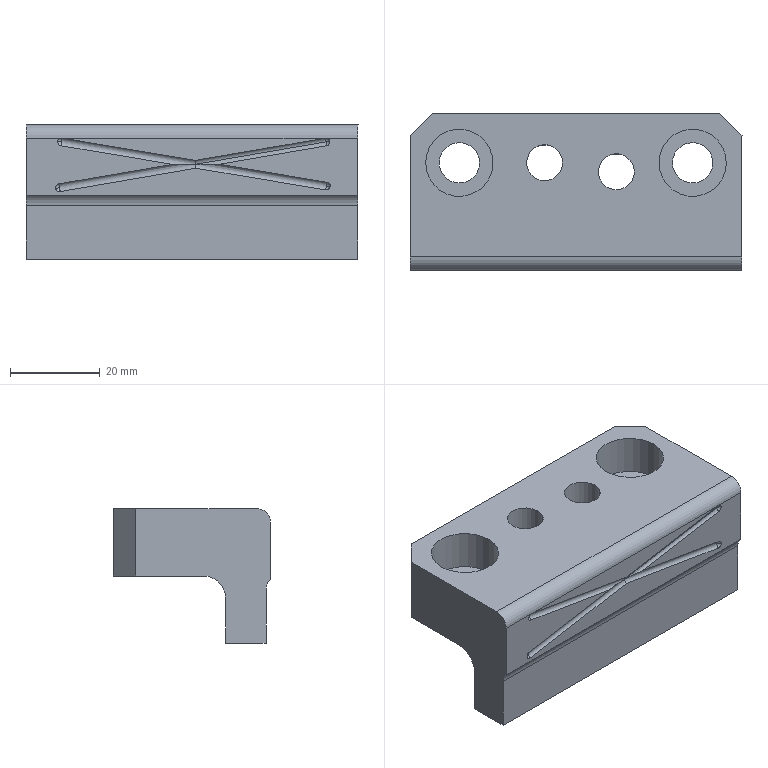Part | CATIA | 1 solid | 42 faces | box 74 x 35 x 30 mm | volume 43302 mm3 | cylinder 20 | plane 14 | sphere 8 | commonest cylinder face diameters 2 x5 8 x4 9 x4 15 x4 6 x2 10 x1
STEP:
#1=CARTESIAN_POINT('',(-37.,5.,-15.));
#2=VERTEX_POINT('',#1);
#3=CARTESIAN_POINT('',(37.,5.,-15.));
#4=VERTEX_POINT('',#3);
#5=CARTESIAN_POINT('',(0.,5.,-15.));
#6=DIRECTION('',(1.,0.,0.));
#7=VECTOR('',#6,1.);
#8=LINE('',#5,#7);
#9=EDGE_CURVE('',#2,#4,#8,.T.);
#10=ORIENTED_EDGE('',*,*,#9,.T.);
#11=CARTESIAN_POINT('',(37.,0.,-20.));
#12=VERTEX_POINT('',#11);
#13=CARTESIAN_POINT('',(37.,5.,-20.));
#14=DIRECTION('',(1.,0.,0.));
#15=AXIS2_PLACEMENT_3D('',#13,#14,$);
#16=CIRCLE('',#15,5.);
#17=EDGE_CURVE('',#4,#12,#16,.T.);
#18=ORIENTED_EDGE('',*,*,#17,.T.);
#19=CARTESIAN_POINT('',(-37.,0.,-20.));
#20=VERTEX_POINT('',#19);
#21=CARTESIAN_POINT('',(0.,0.,-20.));
#22=DIRECTION('',(1.,0.,0.));
#23=VECTOR('',#22,1.);
#24=LINE('',#21,#23);
#25=EDGE_CURVE('',#20,#12,#24,.T.);
#26=ORIENTED_EDGE('',*,*,#25,.F.);
#27=CARTESIAN_POINT('',(-37.,5.,-20.));
#28=DIRECTION('',(1.,0.,0.));
#29=AXIS2_PLACEMENT_3D('',#27,#28,$);
#30=CIRCLE('',#29,5.);
#31=EDGE_CURVE('',#20,#2,#30,.F.);
#32=ORIENTED_EDGE('',*,*,#31,.T.);
#33=EDGE_LOOP('',(#10,#18,#26,#32));
#34=FACE_OUTER_BOUND('',#33,.T.);
#35=CARTESIAN_POINT('',(0.,5.,-20.));
#36=DIRECTION('',(1.,0.,0.));
#37=DIRECTION('',(0.,0.,1.));
#38=AXIS2_PLACEMENT_3D('',#35,#36,#37);
#39=CYLINDRICAL_SURFACE('',#38,5.);
#40=ADVANCED_FACE('',(#34),#39,.F.);
#41=CARTESIAN_POINT('',(-37.,0.,-30.));
#42=VERTEX_POINT('',#41);
#43=CARTESIAN_POINT('',(-37.,0.,-25.));
#44=DIRECTION('',(0.,0.,1.));
#45=VECTOR('',#44,1.);
#46=LINE('',#43,#45);
#47=EDGE_CURVE('',#42,#20,#46,.T.);
#48=ORIENTED_EDGE('',*,*,#47,.T.);
#49=ORIENTED_EDGE('',*,*,#25,.T.);
#50=CARTESIAN_POINT('',(37.,0.,-30.));
#51=VERTEX_POINT('',#50);
#52=CARTESIAN_POINT('',(37.,0.,-25.));
#53=DIRECTION('',(0.,0.,1.));
#54=VECTOR('',#53,1.);
#55=LINE('',#52,#54);
#56=EDGE_CURVE('',#51,#12,#55,.T.);
#57=ORIENTED_EDGE('',*,*,#56,.F.);
#58=CARTESIAN_POINT('',(0.,0.,-30.));
#59=DIRECTION('',(1.,0.,0.));
#60=VECTOR('',#59,1.);
#61=LINE('',#58,#60);
#62=EDGE_CURVE('',#42,#51,#61,.T.);
#63=ORIENTED_EDGE('',*,*,#62,.F.);
#64=EDGE_LOOP('',(#48,#49,#57,#63));
#65=FACE_OUTER_BOUND('',#64,.T.);
#66=CARTESIAN_POINT('',(0.,0.,-30.));
#67=DIRECTION('',(0.,1.,0.));
#68=DIRECTION('',(0.,0.,1.));
#69=AXIS2_PLACEMENT_3D('',#66,#67,#68);
#70=PLANE('',#69);
#71=ADVANCED_FACE('',(#65),#70,.T.);
#72=CARTESIAN_POINT('',(-37.,-9.,-30.));
#73=VERTEX_POINT('',#72);
#74=CARTESIAN_POINT('',(-37.,-4.5,-30.));
#75=DIRECTION('',(0.,1.,0.));
#76=VECTOR('',#75,1.);
#77=LINE('',#74,#76);
#78=EDGE_CURVE('',#73,#42,#77,.T.);
#79=ORIENTED_EDGE('',*,*,#78,.T.);
#80=ORIENTED_EDGE('',*,*,#62,.T.);
#81=CARTESIAN_POINT('',(37.,-9.,-30.));
#82=VERTEX_POINT('',#81);
#83=CARTESIAN_POINT('',(37.,-4.5,-30.));
#84=DIRECTION('',(0.,1.,0.));
#85=VECTOR('',#84,1.);
#86=LINE('',#83,#85);
#87=EDGE_CURVE('',#82,#51,#86,.T.);
#88=ORIENTED_EDGE('',*,*,#87,.F.);
#89=CARTESIAN_POINT('',(0.,-9.,-30.));
#90=DIRECTION('',(1.,0.,0.));
#91=VECTOR('',#90,1.);
#92=LINE('',#89,#91);
#93=EDGE_CURVE('',#73,#82,#92,.T.);
#94=ORIENTED_EDGE('',*,*,#93,.F.);
#95=EDGE_LOOP('',(#79,#80,#88,#94));
#96=FACE_OUTER_BOUND('',#95,.T.);
#97=CARTESIAN_POINT('',(0.,-9.,-30.));
#98=DIRECTION('',(0.,0.,-1.));
#99=DIRECTION('',(0.,1.,0.));
#100=AXIS2_PLACEMENT_3D('',#97,#98,#99);
#101=PLANE('',#100);
#102=ADVANCED_FACE('',(#96),#101,.T.);
#103=CARTESIAN_POINT('',(-37.,-9.,-18.));
#104=VERTEX_POINT('',#103);
#105=CARTESIAN_POINT('',(-37.,-9.,-24.));
#106=DIRECTION('',(0.,0.,-1.));
#107=VECTOR('',#106,1.);
#108=LINE('',#105,#107);
#109=EDGE_CURVE('',#104,#73,#108,.T.);
#110=ORIENTED_EDGE('',*,*,#109,.T.);
#111=ORIENTED_EDGE('',*,*,#93,.T.);
#112=CARTESIAN_POINT('',(37.,-9.,-18.));
#113=VERTEX_POINT('',#112);
#114=CARTESIAN_POINT('',(37.,-9.,-24.));
#115=DIRECTION('',(0.,0.,-1.));
#116=VECTOR('',#115,1.);
#117=LINE('',#114,#116);
#118=EDGE_CURVE('',#113,#82,#117,.T.);
#119=ORIENTED_EDGE('',*,*,#118,.F.);
#120=CARTESIAN_POINT('',(0.,-9.,-18.));
#121=DIRECTION('',(1.,0.,0.));
#122=VECTOR('',#121,1.);
#123=LINE('',#120,#122);
#124=EDGE_CURVE('',#104,#113,#123,.T.);
#125=ORIENTED_EDGE('',*,*,#124,.F.);
#126=EDGE_LOOP('',(#110,#111,#119,#125));
#127=FACE_OUTER_BOUND('',#126,.T.);
#128=CARTESIAN_POINT('',(0.,-9.,-18.));
#129=DIRECTION('',(0.,-1.,0.));
#130=DIRECTION('',(0.,0.,-1.));
#131=AXIS2_PLACEMENT_3D('',#128,#129,#130);
#132=PLANE('',#131);
#133=ADVANCED_FACE('',(#127),#132,.T.);
#134=ORIENTED_EDGE('',*,*,#124,.T.);
#135=CARTESIAN_POINT('',(37.,-10.,-15.764));
#136=VERTEX_POINT('',#135);
#137=CARTESIAN_POINT('',(37.,-12.,-18.));
#138=DIRECTION('',(1.,0.,0.));
#139=AXIS2_PLACEMENT_3D('',#137,#138,$);
#140=CIRCLE('',#139,3.);
#141=EDGE_CURVE('',#113,#136,#140,.T.);
#142=ORIENTED_EDGE('',*,*,#141,.T.);
#143=CARTESIAN_POINT('',(-37.,-10.,-15.764));
#144=VERTEX_POINT('',#143);
#145=CARTESIAN_POINT('',(0.,-10.,-15.764));
#146=DIRECTION('',(1.,0.,0.));
#147=VECTOR('',#146,1.);
#148=LINE('',#145,#147);
#149=EDGE_CURVE('',#144,#136,#148,.T.);
#150=ORIENTED_EDGE('',*,*,#149,.F.);
#151=CARTESIAN_POINT('',(-37.,-12.,-18.));
#152=DIRECTION('',(1.,0.,0.));
#153=AXIS2_PLACEMENT_3D('',#151,#152,$);
#154=CIRCLE('',#153,3.);
#155=EDGE_CURVE('',#144,#104,#154,.F.);
#156=ORIENTED_EDGE('',*,*,#155,.T.);
#157=EDGE_LOOP('',(#134,#142,#150,#156));
#158=FACE_OUTER_BOUND('',#157,.T.);
#159=CARTESIAN_POINT('',(0.,-12.,-18.));
#160=DIRECTION('',(1.,0.,0.));
#161=DIRECTION('',(0.,1.,0.));
#162=AXIS2_PLACEMENT_3D('',#159,#160,#161);
#163=CYLINDRICAL_SURFACE('',#162,3.);
#164=ADVANCED_FACE('',(#158),#163,.F.);
#165=CARTESIAN_POINT('',(37.,20.,0.));
#166=VERTEX_POINT('',#165);
#167=CARTESIAN_POINT('',(37.,-7.,0.));
#168=VERTEX_POINT('',#167);
#169=CARTESIAN_POINT('',(37.,6.5,0.));
#170=DIRECTION('',(0.,-1.,0.));
#171=VECTOR('',#170,1.);
#172=LINE('',#169,#171);
#173=EDGE_CURVE('',#166,#168,#172,.T.);
#174=ORIENTED_EDGE('',*,*,#173,.T.);
#175=CARTESIAN_POINT('',(37.,-10.,-3.));
#176=VERTEX_POINT('',#175);
#177=CARTESIAN_POINT('',(37.,-7.,-3.));
#178=DIRECTION('',(1.,0.,0.));
#179=AXIS2_PLACEMENT_3D('',#177,#178,$);
#180=CIRCLE('',#179,3.);
#181=EDGE_CURVE('',#168,#176,#180,.T.);
#182=ORIENTED_EDGE('',*,*,#181,.T.);
#183=CARTESIAN_POINT('',(37.,-10.,-9.382));
#184=DIRECTION('',(0.,0.,1.));
#185=VECTOR('',#184,1.);
#186=LINE('',#183,#185);
#187=EDGE_CURVE('',#136,#176,#186,.T.);
#188=ORIENTED_EDGE('',*,*,#187,.F.);
#189=ORIENTED_EDGE('',*,*,#141,.F.);
#190=ORIENTED_EDGE('',*,*,#118,.T.);
#191=ORIENTED_EDGE('',*,*,#87,.T.);
#192=ORIENTED_EDGE('',*,*,#56,.T.);
#193=ORIENTED_EDGE('',*,*,#17,.F.);
#194=CARTESIAN_POINT('',(37.,20.,-15.));
#195=VERTEX_POINT('',#194);
#196=CARTESIAN_POINT('',(37.,12.5,-15.));
#197=DIRECTION('',(0.,-1.,0.));
#198=VECTOR('',#197,1.);
#199=LINE('',#196,#198);
#200=EDGE_CURVE('',#195,#4,#199,.T.);
#201=ORIENTED_EDGE('',*,*,#200,.F.);
#202=CARTESIAN_POINT('',(37.,20.,-7.5));
#203=DIRECTION('',(0.,0.,-1.));
#204=VECTOR('',#203,1.);
#205=LINE('',#202,#204);
#206=EDGE_CURVE('',#195,#166,#205,.F.);
#207=ORIENTED_EDGE('',*,*,#206,.T.);
#208=EDGE_LOOP('',(#174,#182,#188,#189,#190,#191,#192,#193,#201,#207));
#209=FACE_OUTER_BOUND('',#208,.T.);
#210=CARTESIAN_POINT('',(37.,-10.,0.));
#211=DIRECTION('',(1.,0.,0.));
#212=DIRECTION('',(0.,1.,0.));
#213=AXIS2_PLACEMENT_3D('',#210,#211,#212);
#214=PLANE('',#213);
#215=ADVANCED_FACE('',(#209),#214,.T.);
#216=ORIENTED_EDGE('',*,*,#206,.F.);
#217=CARTESIAN_POINT('',(32.,25.,-15.));
#218=VERTEX_POINT('',#217);
#219=CARTESIAN_POINT('',(34.5,22.5,-15.));
#220=DIRECTION('',(0.7071,-0.7071,0.));
#221=VECTOR('',#220,1.);
#222=LINE('',#219,#221);
#223=EDGE_CURVE('',#195,#218,#222,.F.);
#224=ORIENTED_EDGE('',*,*,#223,.T.);
#225=CARTESIAN_POINT('',(32.,25.,0.));
#226=VERTEX_POINT('',#225);
#227=CARTESIAN_POINT('',(32.,25.,-15.));
#228=DIRECTION('',(0.,0.,-1.));
#229=VECTOR('',#228,1.);
#230=LINE('',#227,#229);
#231=EDGE_CURVE('',#218,#226,#230,.F.);
#232=ORIENTED_EDGE('',*,*,#231,.T.);
#233=CARTESIAN_POINT('',(34.5,22.5,0.));
#234=DIRECTION('',(0.7071,-0.7071,0.));
#235=VECTOR('',#234,1.);
#236=LINE('',#233,#235);
#237=EDGE_CURVE('',#226,#166,#236,.T.);
#238=ORIENTED_EDGE('',*,*,#237,.T.);
#239=EDGE_LOOP('',(#216,#224,#232,#238));
#240=FACE_OUTER_BOUND('',#239,.T.);
#241=CARTESIAN_POINT('',(32.,25.,6.));
#242=DIRECTION('',(-0.7071,-0.7071,0.));
#243=DIRECTION('',(0.,0.,-1.));
#244=AXIS2_PLACEMENT_3D('',#241,#242,#243);
#245=PLANE('',#244);
#246=ADVANCED_FACE('',(#240),#245,.F.);
#247=CARTESIAN_POINT('',(-37.,20.,-15.));
#248=VERTEX_POINT('',#247);
#249=CARTESIAN_POINT('',(-37.,12.5,-15.));
#250=DIRECTION('',(0.,-1.,0.));
#251=VECTOR('',#250,1.);
#252=LINE('',#249,#251);
#253=EDGE_CURVE('',#248,#2,#252,.T.);
#254=ORIENTED_EDGE('',*,*,#253,.T.);
#255=ORIENTED_EDGE('',*,*,#31,.F.);
#256=ORIENTED_EDGE('',*,*,#47,.F.);
#257=ORIENTED_EDGE('',*,*,#78,.F.);
#258=ORIENTED_EDGE('',*,*,#109,.F.);
#259=ORIENTED_EDGE('',*,*,#155,.F.);
#260=CARTESIAN_POINT('',(-37.,-10.,-3.));
#261=VERTEX_POINT('',#260);
#262=CARTESIAN_POINT('',(-37.,-10.,-9.382));
#263=DIRECTION('',(0.,0.,1.));
#264=VECTOR('',#263,1.);
#265=LINE('',#262,#264);
#266=EDGE_CURVE('',#144,#261,#265,.T.);
#267=ORIENTED_EDGE('',*,*,#266,.T.);
#268=CARTESIAN_POINT('',(-37.,-7.,0.));
#269=VERTEX_POINT('',#268);
#270=CARTESIAN_POINT('',(-37.,-7.,-3.));
#271=DIRECTION('',(-1.,0.,0.));
#272=AXIS2_PLACEMENT_3D('',#270,#271,$);
#273=CIRCLE('',#272,3.);
#274=EDGE_CURVE('',#261,#269,#273,.T.);
#275=ORIENTED_EDGE('',*,*,#274,.T.);
#276=CARTESIAN_POINT('',(-37.,20.,0.));
#277=VERTEX_POINT('',#276);
#278=CARTESIAN_POINT('',(-37.,6.5,0.));
#279=DIRECTION('',(0.,-1.,0.));
#280=VECTOR('',#279,1.);
#281=LINE('',#278,#280);
#282=EDGE_CURVE('',#277,#269,#281,.T.);
#283=ORIENTED_EDGE('',*,*,#282,.F.);
#284=CARTESIAN_POINT('',(-37.,20.,-7.5));
#285=DIRECTION('',(0.,0.,1.));
#286=VECTOR('',#285,1.);
#287=LINE('',#284,#286);
#288=EDGE_CURVE('',#248,#277,#287,.T.);
#289=ORIENTED_EDGE('',*,*,#288,.F.);
#290=EDGE_LOOP('',(#254,#255,#256,#257,#258,#259,#267,#275,#283,#289));
#291=FACE_OUTER_BOUND('',#290,.T.);
#292=CARTESIAN_POINT('',(-37.,25.,0.));
#293=DIRECTION('',(-1.,0.,0.));
#294=DIRECTION('',(0.,-1.,0.));
#295=AXIS2_PLACEMENT_3D('',#292,#293,#294);
#296=PLANE('',#295);
#297=ADVANCED_FACE('',(#291),#296,.T.);
#298=CARTESIAN_POINT('',(-32.,25.,0.));
#299=VERTEX_POINT('',#298);
#300=CARTESIAN_POINT('',(0.,25.,0.));
#301=DIRECTION('',(1.,0.,0.));
#302=VECTOR('',#301,1.);
#303=LINE('',#300,#302);
#304=EDGE_CURVE('',#299,#226,#303,.T.);
#305=ORIENTED_EDGE('',*,*,#304,.T.);
#306=ORIENTED_EDGE('',*,*,#231,.F.);
#307=CARTESIAN_POINT('',(-32.,25.,-15.));
#308=VERTEX_POINT('',#307);
#309=CARTESIAN_POINT('',(0.,25.,-15.));
#310=DIRECTION('',(1.,0.,0.));
#311=VECTOR('',#310,1.);
#312=LINE('',#309,#311);
#313=EDGE_CURVE('',#308,#218,#312,.T.);
#314=ORIENTED_EDGE('',*,*,#313,.F.);
#315=CARTESIAN_POINT('',(-32.,25.,-7.5));
#316=DIRECTION('',(0.,0.,1.));
#317=VECTOR('',#316,1.);
#318=LINE('',#315,#317);
#319=EDGE_CURVE('',#308,#299,#318,.T.);
#320=ORIENTED_EDGE('',*,*,#319,.T.);
#321=EDGE_LOOP('',(#305,#306,#314,#320));
#322=FACE_OUTER_BOUND('',#321,.T.);
#323=CARTESIAN_POINT('',(0.,25.,-15.));
#324=DIRECTION('',(0.,1.,0.));
#325=DIRECTION('',(0.,0.,1.));
#326=AXIS2_PLACEMENT_3D('',#323,#324,#325);
#327=PLANE('',#326);
#328=ADVANCED_FACE('',(#322),#327,.T.);
#329=ORIENTED_EDGE('',*,*,#319,.F.);
#330=CARTESIAN_POINT('',(-34.5,22.5,-15.));
#331=DIRECTION('',(-0.7071,-0.7071,0.));
#332=VECTOR('',#331,1.);
#333=LINE('',#330,#332);
#334=EDGE_CURVE('',#308,#248,#333,.T.);
#335=ORIENTED_EDGE('',*,*,#334,.T.);
#336=ORIENTED_EDGE('',*,*,#288,.T.);
#337=CARTESIAN_POINT('',(-34.5,22.5,0.));
#338=DIRECTION('',(-0.7071,-0.7071,0.));
#339=VECTOR('',#338,1.);
#340=LINE('',#337,#339);
#341=EDGE_CURVE('',#277,#299,#340,.F.);
#342=ORIENTED_EDGE('',*,*,#341,.T.);
#343=EDGE_LOOP('',(#329,#335,#336,#342));
#344=FACE_OUTER_BOUND('',#343,.T.);
#345=CARTESIAN_POINT('',(-32.,25.,-36.));
#346=DIRECTION('',(0.7071,-0.7071,0.));
#347=DIRECTION('',(0.,0.,1.));
#348=AXIS2_PLACEMENT_3D('',#345,#346,#347);
#349=PLANE('',#348);
#350=ADVANCED_FACE('',(#344),#349,.F.);
#351=CARTESIAN_POINT('',(-28.849,-10.,-3.));
#352=VERTEX_POINT('',#351);
#353=CARTESIAN_POINT('',(29.662,-10.,-3.));
#354=VERTEX_POINT('',#353);
#355=CARTESIAN_POINT('',(0.4066,-10.,-3.));
#356=DIRECTION('',(1.,0.,0.));
#357=VECTOR('',#356,1.);
#358=LINE('',#355,#357);
#359=EDGE_CURVE('',#352,#354,#358,.T.);
#360=ORIENTED_EDGE('',*,*,#359,.F.);
#361=CARTESIAN_POINT('',(0.8431,-10.,-7.948));
#362=VERTEX_POINT('',#361);
#363=CARTESIAN_POINT('',(-14.003,-10.,-5.474));
#364=DIRECTION('',(-0.9864,0.,0.1644));
#365=VECTOR('',#364,1.);
#366=LINE('',#363,#365);
#367=EDGE_CURVE('',#362,#352,#366,.T.);
#368=ORIENTED_EDGE('',*,*,#367,.F.);
#369=CARTESIAN_POINT('',(15.253,-10.,-5.474));
#370=DIRECTION('',(0.9856,0.,0.1692));
#371=VECTOR('',#370,1.);
#372=LINE('',#369,#371);
#373=EDGE_CURVE('',#362,#354,#372,.T.);
#374=ORIENTED_EDGE('',*,*,#373,.T.);
#375=EDGE_LOOP('',(#360,#368,#374));
#376=FACE_OUTER_BOUND('',#375,.T.);
#377=CARTESIAN_POINT('',(0.,-10.,-3.));
#378=DIRECTION('',(0.,-1.,0.));
#379=DIRECTION('',(0.,0.,-1.));
#380=AXIS2_PLACEMENT_3D('',#377,#378,#379);
#381=PLANE('',#380);
#382=ADVANCED_FACE('',(#376),#381,.T.);
#383=CARTESIAN_POINT('',(-29.295,-10.,-3.));
#384=VERTEX_POINT('',#383);
#385=CARTESIAN_POINT('',(-33.147,-10.,-3.));
#386=DIRECTION('',(1.,0.,0.));
#387=VECTOR('',#386,1.);
#388=LINE('',#385,#387);
#389=EDGE_CURVE('',#261,#384,#388,.T.);
#390=ORIENTED_EDGE('',*,*,#389,.F.);
#391=ORIENTED_EDGE('',*,*,#266,.F.);
#392=ORIENTED_EDGE('',*,*,#149,.T.);
#393=ORIENTED_EDGE('',*,*,#187,.T.);
#394=CARTESIAN_POINT('',(30.057,-10.,-3.));
#395=VERTEX_POINT('',#394);
#396=CARTESIAN_POINT('',(33.528,-10.,-3.));
#397=DIRECTION('',(1.,0.,0.));
#398=VECTOR('',#397,1.);
#399=LINE('',#396,#398);
#400=EDGE_CURVE('',#395,#176,#399,.T.);
#401=ORIENTED_EDGE('',*,*,#400,.F.);
#402=CARTESIAN_POINT('',(30.717,-10.,-3.698));
#403=VERTEX_POINT('',#402);
#404=CARTESIAN_POINT('',(30.717,-10.,-3.698));
#405=CARTESIAN_POINT('',(30.701,-10.,-3.603));
#406=CARTESIAN_POINT('',(30.672,-10.,-3.511));
#407=CARTESIAN_POINT('',(30.63,-10.,-3.424));
#408=CARTESIAN_POINT('',(30.558,-10.,-3.315));
#409=CARTESIAN_POINT('',(30.468,-10.,-3.223));
#410=CARTESIAN_POINT('',(30.444,-10.,-3.2));
#411=CARTESIAN_POINT('',(30.36,-10.,-3.129));
#412=CARTESIAN_POINT('',(30.268,-10.,-3.073));
#413=CARTESIAN_POINT('',(30.201,-10.,-3.042));
#414=CARTESIAN_POINT('',(30.132,-10.,-3.018));
#415=CARTESIAN_POINT('',(30.067,-10.,-3.002));
#416=CARTESIAN_POINT('',(30.064,-10.,-3.002));
#417=CARTESIAN_POINT('',(30.06,-10.,-3.001));
#418=CARTESIAN_POINT('',(30.057,-10.,-3.));
#419=B_SPLINE_CURVE_WITH_KNOTS('',5,(#404,#405,#406,#407,#408,#409,#410,#411,#412,#413,#414,#415,#416,#417,#418),.UNSPECIFIED.,.F.,.U.,(6,3,3,3,6),(0.,0.6764,0.913,1.466,1.496),.UNSPECIFIED.);
#420=EDGE_CURVE('',#403,#395,#419,.T.);
#421=ORIENTED_EDGE('',*,*,#420,.F.);
#422=CARTESIAN_POINT('',(30.01,-10.,-4.698));
#423=VERTEX_POINT('',#422);
#424=CARTESIAN_POINT('',(30.01,-10.,-4.698));
#425=CARTESIAN_POINT('',(30.057,-10.,-4.69));
#426=CARTESIAN_POINT('',(30.104,-10.,-4.678));
#427=CARTESIAN_POINT('',(30.152,-10.,-4.663));
#428=CARTESIAN_POINT('',(30.24,-10.,-4.629));
#429=CARTESIAN_POINT('',(30.332,-10.,-4.575));
#430=CARTESIAN_POINT('',(30.373,-10.,-4.547));
#431=CARTESIAN_POINT('',(30.442,-10.,-4.493));
#432=CARTESIAN_POINT('',(30.507,-10.,-4.425));
#433=CARTESIAN_POINT('',(30.532,-10.,-4.397));
#434=CARTESIAN_POINT('',(30.598,-10.,-4.312));
#435=CARTESIAN_POINT('',(30.651,-10.,-4.216));
#436=CARTESIAN_POINT('',(30.678,-10.,-4.151));
#437=CARTESIAN_POINT('',(30.718,-10.,-4.022));
#438=CARTESIAN_POINT('',(30.732,-10.,-3.888));
#439=CARTESIAN_POINT('',(30.733,-10.,-3.824));
#440=CARTESIAN_POINT('',(30.728,-10.,-3.76));
#441=CARTESIAN_POINT('',(30.717,-10.,-3.698));
#442=B_SPLINE_CURVE_WITH_KNOTS('',5,(#424,#425,#426,#427,#428,#429,#430,#431,#432,#433,#434,#435,#436,#437,#438,#439,#440,#441),.UNSPECIFIED.,.F.,.U.,(6,3,3,3,3,6),(0.,0.5372,0.9589,1.243,1.741,2.191),.UNSPECIFIED.);
#443=EDGE_CURVE('',#423,#403,#442,.T.);
#444=ORIENTED_EDGE('',*,*,#443,.F.);
#445=CARTESIAN_POINT('',(6.037,-10.,-8.814));
#446=VERTEX_POINT('',#445);
#447=CARTESIAN_POINT('',(18.024,-10.,-6.756));
#448=DIRECTION('',(-0.9856,0.,-0.1692));
#449=VECTOR('',#448,1.);
#450=LINE('',#447,#449);
#451=EDGE_CURVE('',#423,#446,#450,.T.);
#452=ORIENTED_EDGE('',*,*,#451,.T.);
#453=CARTESIAN_POINT('',(30.078,-10.,-12.821));
#454=VERTEX_POINT('',#453);
#455=CARTESIAN_POINT('',(18.058,-10.,-10.817));
#456=DIRECTION('',(0.9864,0.,-0.1644));
#457=VECTOR('',#456,1.);
#458=LINE('',#455,#457);
#459=EDGE_CURVE('',#446,#454,#458,.T.);
#460=ORIENTED_EDGE('',*,*,#459,.T.);
#461=CARTESIAN_POINT('',(30.79,-10.,-13.817));
#462=VERTEX_POINT('',#461);
#463=CARTESIAN_POINT('',(30.078,-10.,-12.821));
#464=CARTESIAN_POINT('',(30.126,-10.,-12.829));
#465=CARTESIAN_POINT('',(30.173,-10.,-12.84));
#466=CARTESIAN_POINT('',(30.22,-10.,-12.855));
#467=CARTESIAN_POINT('',(30.308,-10.,-12.889));
#468=CARTESIAN_POINT('',(30.401,-10.,-12.942));
#469=CARTESIAN_POINT('',(30.442,-10.,-12.969));
#470=CARTESIAN_POINT('',(30.512,-10.,-13.024));
#471=CARTESIAN_POINT('',(30.577,-10.,-13.091));
#472=CARTESIAN_POINT('',(30.602,-10.,-13.119));
#473=CARTESIAN_POINT('',(30.668,-10.,-13.204));
#474=CARTESIAN_POINT('',(30.721,-10.,-13.3));
#475=CARTESIAN_POINT('',(30.749,-10.,-13.365));
#476=CARTESIAN_POINT('',(30.789,-10.,-13.493));
#477=CARTESIAN_POINT('',(30.804,-10.,-13.627));
#478=CARTESIAN_POINT('',(30.806,-10.,-13.691));
#479=CARTESIAN_POINT('',(30.801,-10.,-13.755));
#480=CARTESIAN_POINT('',(30.79,-10.,-13.817));
#481=B_SPLINE_CURVE_WITH_KNOTS('',5,(#463,#464,#465,#466,#467,#468,#469,#470,#471,#472,#473,#474,#475,#476,#477,#478,#479,#480),.UNSPECIFIED.,.F.,.U.,(6,3,3,3,3,6),(0.,0.5372,0.9589,1.243,1.741,2.191),.UNSPECIFIED.);
#482=EDGE_CURVE('',#454,#462,#481,.T.);
#483=ORIENTED_EDGE('',*,*,#482,.T.);
#484=CARTESIAN_POINT('',(29.794,-10.,-14.529));
#485=VERTEX_POINT('',#484);
#486=CARTESIAN_POINT('',(29.794,-10.,-14.529));
#487=CARTESIAN_POINT('',(29.841,-10.,-14.537));
#488=CARTESIAN_POINT('',(29.889,-10.,-14.542));
#489=CARTESIAN_POINT('',(29.939,-10.,-14.543));
#490=CARTESIAN_POINT('',(30.033,-10.,-14.539));
#491=CARTESIAN_POINT('',(30.138,-10.,-14.519));
#492=CARTESIAN_POINT('',(30.186,-10.,-14.507));
#493=CARTESIAN_POINT('',(30.269,-10.,-14.478));
#494=CARTESIAN_POINT('',(30.353,-10.,-14.436));
#495=CARTESIAN_POINT('',(30.386,-10.,-14.417));
#496=CARTESIAN_POINT('',(30.475,-10.,-14.358));
#497=CARTESIAN_POINT('',(30.557,-10.,-14.285));
#498=CARTESIAN_POINT('',(30.605,-10.,-14.232));
#499=CARTESIAN_POINT('',(30.684,-10.,-14.124));
#500=CARTESIAN_POINT('',(30.742,-10.,-14.002));
#501=CARTESIAN_POINT('',(30.764,-10.,-13.942));
#502=CARTESIAN_POINT('',(30.78,-10.,-13.88));
#503=CARTESIAN_POINT('',(30.79,-10.,-13.817));
#504=B_SPLINE_CURVE_WITH_KNOTS('',5,(#486,#487,#488,#489,#490,#491,#492,#493,#494,#495,#496,#497,#498,#499,#500,#501,#502,#503),.UNSPECIFIED.,.F.,.U.,(6,3,3,3,3,6),(0.,0.5372,0.9589,1.243,1.741,2.191),.UNSPECIFIED.);
#505=EDGE_CURVE('',#485,#462,#504,.T.);
#506=ORIENTED_EDGE('',*,*,#505,.F.);
#507=CARTESIAN_POINT('',(0.8474,-10.,-9.705));
#508=VERTEX_POINT('',#507);
#509=CARTESIAN_POINT('',(15.321,-10.,-12.117));
#510=DIRECTION('',(0.9864,0.,-0.1644));
#511=VECTOR('',#510,1.);
#512=LINE('',#509,#511);
#513=EDGE_CURVE('',#508,#485,#512,.T.);
#514=ORIENTED_EDGE('',*,*,#513,.F.);
#515=CARTESIAN_POINT('',(-29.376,-10.,-14.895));
#516=VERTEX_POINT('',#515);
#517=CARTESIAN_POINT('',(-14.264,-10.,-12.3));
#518=DIRECTION('',(-0.9856,0.,-0.1692));
#519=VECTOR('',#518,1.);
#520=LINE('',#517,#519);
#521=EDGE_CURVE('',#508,#516,#520,.T.);
#522=ORIENTED_EDGE('',*,*,#521,.T.);
#523=CARTESIAN_POINT('',(-30.376,-10.,-14.188));
#524=VERTEX_POINT('',#523);
#525=CARTESIAN_POINT('',(-29.376,-10.,-14.895));
#526=CARTESIAN_POINT('',(-29.423,-10.,-14.903));
#527=CARTESIAN_POINT('',(-29.471,-10.,-14.908));
#528=CARTESIAN_POINT('',(-29.521,-10.,-14.909));
#529=CARTESIAN_POINT('',(-29.615,-10.,-14.906));
#530=CARTESIAN_POINT('',(-29.72,-10.,-14.886));
#531=CARTESIAN_POINT('',(-29.768,-10.,-14.874));
#532=CARTESIAN_POINT('',(-29.852,-10.,-14.845));
#533=CARTESIAN_POINT('',(-29.935,-10.,-14.804));
#534=CARTESIAN_POINT('',(-29.969,-10.,-14.785));
#535=CARTESIAN_POINT('',(-30.058,-10.,-14.727));
#536=CARTESIAN_POINT('',(-30.14,-10.,-14.654));
#537=CARTESIAN_POINT('',(-30.188,-10.,-14.602));
#538=CARTESIAN_POINT('',(-30.268,-10.,-14.494));
#539=CARTESIAN_POINT('',(-30.326,-10.,-14.372));
#540=CARTESIAN_POINT('',(-30.349,-10.,-14.312));
#541=CARTESIAN_POINT('',(-30.365,-10.,-14.25));
#542=CARTESIAN_POINT('',(-30.376,-10.,-14.188));
#543=B_SPLINE_CURVE_WITH_KNOTS('',5,(#525,#526,#527,#528,#529,#530,#531,#532,#533,#534,#535,#536,#537,#538,#539,#540,#541,#542),.UNSPECIFIED.,.F.,.U.,(6,3,3,3,3,6),(0.,0.5372,0.9589,1.243,1.741,2.191),.UNSPECIFIED.);
#544=EDGE_CURVE('',#516,#524,#543,.T.);
#545=ORIENTED_EDGE('',*,*,#544,.T.);
#546=CARTESIAN_POINT('',(-29.669,-10.,-13.188));
#547=VERTEX_POINT('',#546);
#548=CARTESIAN_POINT('',(-29.669,-10.,-13.188));
#549=CARTESIAN_POINT('',(-29.716,-10.,-13.196));
#550=CARTESIAN_POINT('',(-29.763,-10.,-13.207));
#551=CARTESIAN_POINT('',(-29.811,-10.,-13.222));
#552=CARTESIAN_POINT('',(-29.898,-10.,-13.257));
#553=CARTESIAN_POINT('',(-29.991,-10.,-13.31));
#554=CARTESIAN_POINT('',(-30.032,-10.,-13.338));
#555=CARTESIAN_POINT('',(-30.101,-10.,-13.393));
#556=CARTESIAN_POINT('',(-30.166,-10.,-13.46));
#557=CARTESIAN_POINT('',(-30.191,-10.,-13.489));
#558=CARTESIAN_POINT('',(-30.256,-10.,-13.573));
#559=CARTESIAN_POINT('',(-30.309,-10.,-13.67));
#560=CARTESIAN_POINT('',(-30.337,-10.,-13.735));
#561=CARTESIAN_POINT('',(-30.377,-10.,-13.863));
#562=CARTESIAN_POINT('',(-30.391,-10.,-13.997));
#563=CARTESIAN_POINT('',(-30.392,-10.,-14.061));
#564=CARTESIAN_POINT('',(-30.387,-10.,-14.125));
#565=CARTESIAN_POINT('',(-30.376,-10.,-14.188));
#566=B_SPLINE_CURVE_WITH_KNOTS('',5,(#548,#549,#550,#551,#552,#553,#554,#555,#556,#557,#558,#559,#560,#561,#562,#563,#564,#565),.UNSPECIFIED.,.F.,.U.,(6,3,3,3,3,6),(0.,0.5372,0.9589,1.243,1.741,2.191),.UNSPECIFIED.);
#567=EDGE_CURVE('',#547,#524,#566,.T.);
#568=ORIENTED_EDGE('',*,*,#567,.F.);
#569=CARTESIAN_POINT('',(-4.346,-10.,-8.84));
#570=VERTEX_POINT('',#569);
#571=CARTESIAN_POINT('',(-17.008,-10.,-11.014));
#572=DIRECTION('',(-0.9856,0.,-0.1692));
#573=VECTOR('',#572,1.);
#574=LINE('',#571,#573);
#575=EDGE_CURVE('',#570,#547,#574,.T.);
#576=ORIENTED_EDGE('',*,*,#575,.F.);
#577=CARTESIAN_POINT('',(-29.224,-10.,-4.694));
#578=VERTEX_POINT('',#577);
#579=CARTESIAN_POINT('',(-16.785,-10.,-6.767));
#580=DIRECTION('',(0.9864,0.,-0.1644));
#581=VECTOR('',#580,1.);
#582=LINE('',#579,#581);
#583=EDGE_CURVE('',#578,#570,#582,.T.);
#584=ORIENTED_EDGE('',*,*,#583,.F.);
#585=CARTESIAN_POINT('',(-29.935,-10.,-3.697));
#586=VERTEX_POINT('',#585);
#587=CARTESIAN_POINT('',(-29.224,-10.,-4.694));
#588=CARTESIAN_POINT('',(-29.271,-10.,-4.686));
#589=CARTESIAN_POINT('',(-29.318,-10.,-4.674));
#590=CARTESIAN_POINT('',(-29.365,-10.,-4.66));
#591=CARTESIAN_POINT('',(-29.453,-10.,-4.626));
#592=CARTESIAN_POINT('',(-29.546,-10.,-4.572));
#593=CARTESIAN_POINT('',(-29.587,-10.,-4.545));
#594=CARTESIAN_POINT('',(-29.657,-10.,-4.491));
#595=CARTESIAN_POINT('',(-29.722,-10.,-4.424));
#596=CARTESIAN_POINT('',(-29.747,-10.,-4.395));
#597=CARTESIAN_POINT('',(-29.813,-10.,-4.311));
#598=CARTESIAN_POINT('',(-29.866,-10.,-4.215));
#599=CARTESIAN_POINT('',(-29.894,-10.,-4.15));
#600=CARTESIAN_POINT('',(-29.935,-10.,-4.021));
#601=CARTESIAN_POINT('',(-29.949,-10.,-3.888));
#602=CARTESIAN_POINT('',(-29.951,-10.,-3.824));
#603=CARTESIAN_POINT('',(-29.946,-10.,-3.76));
#604=CARTESIAN_POINT('',(-29.935,-10.,-3.697));
#605=B_SPLINE_CURVE_WITH_KNOTS('',5,(#587,#588,#589,#590,#591,#592,#593,#594,#595,#596,#597,#598,#599,#600,#601,#602,#603,#604),.UNSPECIFIED.,.F.,.U.,(6,3,3,3,3,6),(0.,0.5372,0.9589,1.243,1.741,2.191),.UNSPECIFIED.);
#606=EDGE_CURVE('',#578,#586,#605,.T.);
#607=ORIENTED_EDGE('',*,*,#606,.T.);
#608=CARTESIAN_POINT('',(-29.935,-10.,-3.697));
#609=CARTESIAN_POINT('',(-29.92,-10.,-3.603));
#610=CARTESIAN_POINT('',(-29.891,-10.,-3.51));
#611=CARTESIAN_POINT('',(-29.85,-10.,-3.423));
#612=CARTESIAN_POINT('',(-29.778,-10.,-3.314));
#613=CARTESIAN_POINT('',(-29.689,-10.,-3.221));
#614=CARTESIAN_POINT('',(-29.665,-10.,-3.198));
#615=CARTESIAN_POINT('',(-29.581,-10.,-3.127));
#616=CARTESIAN_POINT('',(-29.489,-10.,-3.07));
#617=CARTESIAN_POINT('',(-29.423,-10.,-3.039));
#618=CARTESIAN_POINT('',(-29.357,-10.,-3.016));
#619=CARTESIAN_POINT('',(-29.295,-10.,-3.));
#620=B_SPLINE_CURVE_WITH_KNOTS('',5,(#608,#609,#610,#611,#612,#613,#614,#615,#616,#617,#618,#619),.UNSPECIFIED.,.F.,.U.,(6,3,3,6),(0.,0.6764,0.913,1.467),.UNSPECIFIED.);
#621=EDGE_CURVE('',#586,#384,#620,.T.);
#622=ORIENTED_EDGE('',*,*,#621,.T.);
#623=EDGE_LOOP('',(#390,#391,#392,#393,#401,#421,#444,#452,#460,#483,#506,#514,#522,#545,#568,#576,#584,#607,#622));
#624=FACE_OUTER_BOUND('',#623,.T.);
#625=ADVANCED_FACE('',(#624),#381,.T.);
#626=ORIENTED_EDGE('',*,*,#359,.T.);
#627=CARTESIAN_POINT('',(29.717,-10.,-2.991));
#628=VERTEX_POINT('',#627);
#629=CARTESIAN_POINT('',(29.662,-10.,-3.));
#630=CARTESIAN_POINT('',(29.681,-10.,-2.997));
#631=CARTESIAN_POINT('',(29.699,-10.,-2.994));
#632=CARTESIAN_POINT('',(29.717,-10.,-2.991));
#633=B_SPLINE_CURVE_WITH_KNOTS('',3,(#629,#630,#631,#632),.UNSPECIFIED.,.F.,.U.,(4,4),(0.,0.07826),.UNSPECIFIED.);
#634=EDGE_CURVE('',#354,#628,#633,.T.);
#635=ORIENTED_EDGE('',*,*,#634,.T.);
#636=CARTESIAN_POINT('',(30.057,-10.,-3.));
#637=CARTESIAN_POINT('',(29.927,-10.,-2.97));
#638=CARTESIAN_POINT('',(29.819,-10.,-2.973));
#639=CARTESIAN_POINT('',(29.717,-10.,-2.991));
#640=B_SPLINE_CURVE_WITH_KNOTS('',3,(#636,#637,#638,#639),.UNSPECIFIED.,.F.,.U.,(4,4),(0.,0.6959),.UNSPECIFIED.);
#641=EDGE_CURVE('',#395,#628,#640,.T.);
#642=ORIENTED_EDGE('',*,*,#641,.F.);
#643=ORIENTED_EDGE('',*,*,#400,.T.);
#644=ORIENTED_EDGE('',*,*,#181,.F.);
#645=CARTESIAN_POINT('',(0.,-7.,0.));
#646=DIRECTION('',(1.,0.,0.));
#647=VECTOR('',#646,1.);
#648=LINE('',#645,#647);
#649=EDGE_CURVE('',#269,#168,#648,.T.);
#650=ORIENTED_EDGE('',*,*,#649,.F.);
#651=ORIENTED_EDGE('',*,*,#274,.F.);
#652=ORIENTED_EDGE('',*,*,#389,.T.);
#653=CARTESIAN_POINT('',(-28.939,-10.,-2.985));
#654=VERTEX_POINT('',#653);
#655=CARTESIAN_POINT('',(-29.295,-10.,-3.));
#656=CARTESIAN_POINT('',(-29.192,-10.,-2.974));
#657=CARTESIAN_POINT('',(-29.1,-10.,-2.968));
#658=CARTESIAN_POINT('',(-29.019,-10.,-2.972));
#659=CARTESIAN_POINT('',(-28.939,-10.,-2.985));
#660=B_SPLINE_CURVE_WITH_KNOTS('',4,(#655,#656,#657,#658,#659),.UNSPECIFIED.,.F.,.U.,(5,5),(0.,0.7245),.UNSPECIFIED.);
#661=EDGE_CURVE('',#384,#654,#660,.T.);
#662=ORIENTED_EDGE('',*,*,#661,.T.);
#663=CARTESIAN_POINT('',(-28.849,-10.,-3.));
#664=CARTESIAN_POINT('',(-28.879,-10.,-2.995));
#665=CARTESIAN_POINT('',(-28.909,-10.,-2.99));
#666=CARTESIAN_POINT('',(-28.939,-10.,-2.985));
#667=B_SPLINE_CURVE_WITH_KNOTS('',3,(#663,#664,#665,#666),.UNSPECIFIED.,.F.,.U.,(4,4),(0.,0.1283),.UNSPECIFIED.);
#668=EDGE_CURVE('',#352,#654,#667,.T.);
#669=ORIENTED_EDGE('',*,*,#668,.F.);
#670=EDGE_LOOP('',(#626,#635,#642,#643,#644,#650,#651,#652,#662,#669));
#671=FACE_OUTER_BOUND('',#670,.T.);
#672=CARTESIAN_POINT('',(0.,-7.,-3.));
#673=DIRECTION('',(1.,0.,0.));
#674=DIRECTION('',(0.,0.,1.));
#675=AXIS2_PLACEMENT_3D('',#672,#673,#674);
#676=CYLINDRICAL_SURFACE('',#675,3.);
#677=ADVANCED_FACE('',(#671),#676,.T.);
#678=CARTESIAN_POINT('',(-29.081,-9.5,-3.839));
#679=VERTEX_POINT('',#678);
#680=CARTESIAN_POINT('',(-29.081,-10.5,-3.839));
#681=DIRECTION('',(0.9864,0.,-0.1644));
#682=AXIS2_PLACEMENT_3D('',#680,#681,$);
#683=CIRCLE('',#682,1.);
#684=EDGE_CURVE('',#679,#654,#683,.T.);
#685=ORIENTED_EDGE('',*,*,#684,.F.);
#686=CARTESIAN_POINT('',(-29.081,-10.5,-3.839));
#687=DIRECTION('',(0.9864,0.,-0.1644));
#688=AXIS2_PLACEMENT_3D('',#686,#687,$);
#689=CIRCLE('',#688,1.);
#690=EDGE_CURVE('',#578,#679,#689,.T.);
#691=ORIENTED_EDGE('',*,*,#690,.F.);
#692=ORIENTED_EDGE('',*,*,#583,.T.);
#693=CARTESIAN_POINT('',(0.8453,-9.5,-8.827));
#694=VERTEX_POINT('',#693);
#695=CARTESIAN_POINT('',(-4.346,-10.,-8.84));
#696=CARTESIAN_POINT('',(-4.09,-9.926,-8.839));
#697=CARTESIAN_POINT('',(-3.815,-9.865,-8.838));
#698=CARTESIAN_POINT('',(-3.555,-9.816,-8.838));
#699=CARTESIAN_POINT('',(-2.808,-9.696,-8.836));
#700=CARTESIAN_POINT('',(-2.055,-9.618,-8.834));
#701=CARTESIAN_POINT('',(-1.587,-9.58,-8.833));
#702=CARTESIAN_POINT('',(-0.9217,-9.54,-8.831));
#703=CARTESIAN_POINT('',(-0.2557,-9.516,-8.83));
#704=CARTESIAN_POINT('',(-0.07302,-9.511,-8.829));
#705=CARTESIAN_POINT('',(0.2404,-9.504,-8.828));
#706=CARTESIAN_POINT('',(0.5539,-9.501,-8.828));
#707=CARTESIAN_POINT('',(0.5839,-9.501,-8.827));
#708=CARTESIAN_POINT('',(0.7146,-9.5,-8.827));
#709=CARTESIAN_POINT('',(0.8453,-9.5,-8.827));
#710=B_SPLINE_CURVE_WITH_KNOTS('',5,(#695,#696,#697,#698,#699,#700,#701,#702,#703,#704,#705,#706,#707,#708,#709),.UNSPECIFIED.,.F.,.U.,(6,3,3,3,6),(1.42,3.35,6.769,8.062,8.986),.UNSPECIFIED.);
#711=EDGE_CURVE('',#570,#694,#710,.T.);
#712=ORIENTED_EDGE('',*,*,#711,.T.);
#713=CARTESIAN_POINT('',(0.8431,-10.,-7.948));
#714=CARTESIAN_POINT('',(0.8435,-9.772,-8.082));
#715=CARTESIAN_POINT('',(0.844,-9.591,-8.297));
#716=CARTESIAN_POINT('',(0.8446,-9.5,-8.562));
#717=CARTESIAN_POINT('',(0.8453,-9.5,-8.827));
#718=B_SPLINE_CURVE_WITH_KNOTS('',4,(#713,#714,#715,#716,#717),.UNSPECIFIED.,.F.,.U.,(5,5),(0.7416,2.238),.UNSPECIFIED.);
#719=EDGE_CURVE('',#694,#362,#718,.F.);
#720=ORIENTED_EDGE('',*,*,#719,.T.);
#721=ORIENTED_EDGE('',*,*,#367,.T.);
#722=ORIENTED_EDGE('',*,*,#668,.T.);
#723=EDGE_LOOP('',(#685,#691,#692,#712,#720,#721,#722));
#724=FACE_OUTER_BOUND('',#723,.T.);
#725=CARTESIAN_POINT('',(-0.2883,-10.5,-8.638));
#726=DIRECTION('',(0.9864,0.,-0.1644));
#727=DIRECTION('',(-0.1644,0.,-0.9864));
#728=AXIS2_PLACEMENT_3D('',#725,#726,#727);
#729=CYLINDRICAL_SURFACE('',#728,1.);
#730=ADVANCED_FACE('',(#724),#729,.F.);
#731=ORIENTED_EDGE('',*,*,#634,.F.);
#732=ORIENTED_EDGE('',*,*,#373,.F.);
#733=ORIENTED_EDGE('',*,*,#719,.F.);
#734=CARTESIAN_POINT('',(29.864,-9.5,-3.844));
#735=VERTEX_POINT('',#734);
#736=CARTESIAN_POINT('',(14.433,-9.5,-6.494));
#737=DIRECTION('',(0.9856,0.,0.1692));
#738=VECTOR('',#737,1.);
#739=LINE('',#736,#738);
#740=EDGE_CURVE('',#694,#735,#739,.T.);
#741=ORIENTED_EDGE('',*,*,#740,.T.);
#742=CARTESIAN_POINT('',(29.864,-10.5,-3.844));
#743=DIRECTION('',(0.9856,0.,0.1692));
#744=AXIS2_PLACEMENT_3D('',#742,#743,$);
#745=CIRCLE('',#744,1.);
#746=EDGE_CURVE('',#735,#628,#745,.T.);
#747=ORIENTED_EDGE('',*,*,#746,.T.);
#748=EDGE_LOOP('',(#731,#732,#733,#741,#747));
#749=FACE_OUTER_BOUND('',#748,.T.);
#750=CARTESIAN_POINT('',(14.433,-10.5,-6.494));
#751=DIRECTION('',(0.9856,0.,0.1692));
#752=DIRECTION('',(0.,1.,0.));
#753=AXIS2_PLACEMENT_3D('',#750,#751,#752);
#754=CYLINDRICAL_SURFACE('',#753,1.);
#755=ADVANCED_FACE('',(#749),#754,.F.);
#756=ORIENTED_EDGE('',*,*,#575,.T.);
#757=CARTESIAN_POINT('',(-29.522,-9.5,-14.041));
#758=VERTEX_POINT('',#757);
#759=CARTESIAN_POINT('',(-29.522,-10.5,-14.041));
#760=DIRECTION('',(-0.9856,0.,-0.1692));
#761=AXIS2_PLACEMENT_3D('',#759,#760,$);
#762=CIRCLE('',#761,1.);
#763=EDGE_CURVE('',#547,#758,#762,.T.);
#764=ORIENTED_EDGE('',*,*,#763,.T.);
#765=CARTESIAN_POINT('',(-29.522,-10.5,-14.041));
#766=DIRECTION('',(-0.9856,0.,-0.1692));
#767=AXIS2_PLACEMENT_3D('',#765,#766,$);
#768=CIRCLE('',#767,1.);
#769=EDGE_CURVE('',#758,#516,#768,.T.);
#770=ORIENTED_EDGE('',*,*,#769,.T.);
#771=ORIENTED_EDGE('',*,*,#521,.F.);
#772=CARTESIAN_POINT('',(0.8474,-10.,-9.705));
#773=CARTESIAN_POINT('',(0.8471,-9.772,-9.572));
#774=CARTESIAN_POINT('',(0.8466,-9.591,-9.357));
#775=CARTESIAN_POINT('',(0.8459,-9.5,-9.091));
#776=CARTESIAN_POINT('',(0.8453,-9.5,-8.827));
#777=B_SPLINE_CURVE_WITH_KNOTS('',4,(#772,#773,#774,#775,#776),.UNSPECIFIED.,.F.,.U.,(5,5),(0.7416,2.238),.UNSPECIFIED.);
#778=EDGE_CURVE('',#508,#694,#777,.T.);
#779=ORIENTED_EDGE('',*,*,#778,.T.);
#780=ORIENTED_EDGE('',*,*,#711,.F.);
#781=EDGE_LOOP('',(#756,#764,#770,#771,#779,#780));
#782=FACE_OUTER_BOUND('',#781,.T.);
#783=CARTESIAN_POINT('',(0.2045,-10.5,-8.937));
#784=DIRECTION('',(-0.9856,0.,-0.1692));
#785=DIRECTION('',(-0.1692,0.,0.9856));
#786=AXIS2_PLACEMENT_3D('',#783,#784,#785);
#787=CYLINDRICAL_SURFACE('',#786,1.);
#788=ADVANCED_FACE('',(#782),#787,.F.);
#789=ORIENTED_EDGE('',*,*,#606,.F.);
#790=ORIENTED_EDGE('',*,*,#690,.T.);
#791=CARTESIAN_POINT('',(-29.081,-10.5,-3.839));
#792=DIRECTION('',(-0.1644,0.,-0.9864));
#793=AXIS2_PLACEMENT_3D('',#791,#792,$);
#794=CIRCLE('',#793,1.);
#795=EDGE_CURVE('',#586,#679,#794,.T.);
#796=ORIENTED_EDGE('',*,*,#795,.F.);
#797=EDGE_LOOP('',(#789,#790,#796));
#798=FACE_OUTER_BOUND('',#797,.T.);
#799=CARTESIAN_POINT('',(-29.081,-10.5,-3.839));
#800=DIRECTION('',(-0.1644,0.,-0.9864));
#801=DIRECTION('',(-0.9528,-0.2588,0.1588));
#802=AXIS2_PLACEMENT_3D('',#799,#800,#801);
#803=SPHERICAL_SURFACE('',#802,1.);
#804=ADVANCED_FACE('',(#798),#803,.F.);
#805=ORIENTED_EDGE('',*,*,#661,.F.);
#806=ORIENTED_EDGE('',*,*,#621,.F.);
#807=ORIENTED_EDGE('',*,*,#795,.T.);
#808=ORIENTED_EDGE('',*,*,#684,.T.);
#809=EDGE_LOOP('',(#805,#806,#807,#808));
#810=FACE_OUTER_BOUND('',#809,.T.);
#811=CARTESIAN_POINT('',(-29.081,-10.5,-3.839));
#812=DIRECTION('',(0.1644,0.,0.9864));
#813=DIRECTION('',(0.2553,0.9659,-0.04255));
#814=AXIS2_PLACEMENT_3D('',#811,#812,#813);
#815=SPHERICAL_SURFACE('',#814,1.);
#816=ADVANCED_FACE('',(#810),#815,.F.);
#817=ORIENTED_EDGE('',*,*,#420,.T.);
#818=ORIENTED_EDGE('',*,*,#641,.T.);
#819=ORIENTED_EDGE('',*,*,#746,.F.);
#820=CARTESIAN_POINT('',(29.864,-10.5,-3.844));
#821=DIRECTION('',(-0.1692,0.,0.9856));
#822=AXIS2_PLACEMENT_3D('',#820,#821,$);
#823=CIRCLE('',#822,1.);
#824=EDGE_CURVE('',#735,#403,#823,.F.);
#825=ORIENTED_EDGE('',*,*,#824,.T.);
#826=EDGE_LOOP('',(#817,#818,#819,#825));
#827=FACE_OUTER_BOUND('',#826,.T.);
#828=CARTESIAN_POINT('',(29.864,-10.5,-3.844));
#829=DIRECTION('',(-0.1692,0.,0.9856));
#830=DIRECTION('',(0.952,-0.2588,0.1635));
#831=AXIS2_PLACEMENT_3D('',#828,#829,#830);
#832=SPHERICAL_SURFACE('',#831,1.);
#833=ADVANCED_FACE('',(#827),#832,.F.);
#834=ORIENTED_EDGE('',*,*,#451,.F.);
#835=CARTESIAN_POINT('',(29.864,-10.5,-3.844));
#836=DIRECTION('',(-0.9856,0.,-0.1692));
#837=AXIS2_PLACEMENT_3D('',#835,#836,$);
#838=CIRCLE('',#837,1.);
#839=EDGE_CURVE('',#423,#735,#838,.F.);
#840=ORIENTED_EDGE('',*,*,#839,.T.);
#841=ORIENTED_EDGE('',*,*,#740,.F.);
#842=CARTESIAN_POINT('',(6.037,-10.,-8.814));
#843=CARTESIAN_POINT('',(5.78,-9.926,-8.815));
#844=CARTESIAN_POINT('',(5.505,-9.865,-8.815));
#845=CARTESIAN_POINT('',(5.246,-9.816,-8.816));
#846=CARTESIAN_POINT('',(4.499,-9.696,-8.818));
#847=CARTESIAN_POINT('',(3.746,-9.618,-8.82));
#848=CARTESIAN_POINT('',(3.278,-9.58,-8.821));
#849=CARTESIAN_POINT('',(2.612,-9.54,-8.822));
#850=CARTESIAN_POINT('',(1.946,-9.516,-8.824));
#851=CARTESIAN_POINT('',(1.764,-9.511,-8.825));
#852=CARTESIAN_POINT('',(1.45,-9.504,-8.825));
#853=CARTESIAN_POINT('',(1.137,-9.501,-8.826));
#854=CARTESIAN_POINT('',(1.107,-9.501,-8.826));
#855=CARTESIAN_POINT('',(0.976,-9.5,-8.826));
#856=CARTESIAN_POINT('',(0.8453,-9.5,-8.827));
#857=B_SPLINE_CURVE_WITH_KNOTS('',5,(#842,#843,#844,#845,#846,#847,#848,#849,#850,#851,#852,#853,#854,#855,#856),.UNSPECIFIED.,.F.,.U.,(6,3,3,3,6),(1.42,3.35,6.769,8.062,8.986),.UNSPECIFIED.);
#858=EDGE_CURVE('',#446,#694,#857,.T.);
#859=ORIENTED_EDGE('',*,*,#858,.F.);
#860=EDGE_LOOP('',(#834,#840,#841,#859));
#861=FACE_OUTER_BOUND('',#860,.T.);
#862=CARTESIAN_POINT('',(13.94,-10.5,-6.578));
#863=DIRECTION('',(-0.9856,0.,-0.1692));
#864=DIRECTION('',(0.,1.,0.));
#865=AXIS2_PLACEMENT_3D('',#862,#863,#864);
#866=CYLINDRICAL_SURFACE('',#865,1.);
#867=ADVANCED_FACE('',(#861),#866,.F.);
#868=ORIENTED_EDGE('',*,*,#513,.T.);
#869=CARTESIAN_POINT('',(29.936,-9.5,-13.675));
#870=VERTEX_POINT('',#869);
#871=CARTESIAN_POINT('',(29.936,-10.5,-13.675));
#872=DIRECTION('',(0.9864,0.,-0.1644));
#873=AXIS2_PLACEMENT_3D('',#871,#872,$);
#874=CIRCLE('',#873,1.);
#875=EDGE_CURVE('',#485,#870,#874,.T.);
#876=ORIENTED_EDGE('',*,*,#875,.T.);
#877=CARTESIAN_POINT('',(29.936,-10.5,-13.675));
#878=DIRECTION('',(0.9864,0.,-0.1644));
#879=AXIS2_PLACEMENT_3D('',#877,#878,$);
#880=CIRCLE('',#879,1.);
#881=EDGE_CURVE('',#870,#454,#880,.T.);
#882=ORIENTED_EDGE('',*,*,#881,.T.);
#883=ORIENTED_EDGE('',*,*,#459,.F.);
#884=ORIENTED_EDGE('',*,*,#858,.T.);
#885=ORIENTED_EDGE('',*,*,#778,.F.);
#886=EDGE_LOOP('',(#868,#876,#882,#883,#884,#885));
#887=FACE_OUTER_BOUND('',#886,.T.);
#888=CARTESIAN_POINT('',(14.45,-10.5,-11.094));
#889=DIRECTION('',(0.9864,0.,-0.1644));
#890=DIRECTION('',(-0.1644,0.,-0.9864));
#891=AXIS2_PLACEMENT_3D('',#888,#889,#890);
#892=CYLINDRICAL_SURFACE('',#891,1.);
#893=ADVANCED_FACE('',(#887),#892,.F.);
#894=ORIENTED_EDGE('',*,*,#544,.F.);
#895=ORIENTED_EDGE('',*,*,#769,.F.);
#896=CARTESIAN_POINT('',(-29.522,-10.5,-14.041));
#897=DIRECTION('',(0.1692,0.,-0.9856));
#898=AXIS2_PLACEMENT_3D('',#896,#897,$);
#899=CIRCLE('',#898,1.);
#900=EDGE_CURVE('',#758,#524,#899,.F.);
#901=ORIENTED_EDGE('',*,*,#900,.T.);
#902=EDGE_LOOP('',(#894,#895,#901));
#903=FACE_OUTER_BOUND('',#902,.T.);
#904=CARTESIAN_POINT('',(-29.522,-10.5,-14.041));
#905=DIRECTION('',(0.1692,0.,-0.9856));
#906=DIRECTION('',(-0.952,-0.2588,-0.1635));
#907=AXIS2_PLACEMENT_3D('',#904,#905,#906);
#908=SPHERICAL_SURFACE('',#907,1.);
#909=ADVANCED_FACE('',(#903),#908,.F.);
#910=ORIENTED_EDGE('',*,*,#567,.T.);
#911=ORIENTED_EDGE('',*,*,#900,.F.);
#912=ORIENTED_EDGE('',*,*,#763,.F.);
#913=EDGE_LOOP('',(#910,#911,#912));
#914=FACE_OUTER_BOUND('',#913,.T.);
#915=CARTESIAN_POINT('',(-29.522,-10.5,-14.041));
#916=DIRECTION('',(-0.1692,0.,0.9856));
#917=DIRECTION('',(0.2551,0.9659,0.0438));
#918=AXIS2_PLACEMENT_3D('',#915,#916,#917);
#919=SPHERICAL_SURFACE('',#918,1.);
#920=ADVANCED_FACE('',(#914),#919,.F.);
#921=ORIENTED_EDGE('',*,*,#443,.T.);
#922=ORIENTED_EDGE('',*,*,#824,.F.);
#923=ORIENTED_EDGE('',*,*,#839,.F.);
#924=EDGE_LOOP('',(#921,#922,#923));
#925=FACE_OUTER_BOUND('',#924,.T.);
#926=CARTESIAN_POINT('',(29.864,-10.5,-3.844));
#927=DIRECTION('',(0.1692,0.,-0.9856));
#928=DIRECTION('',(-0.2551,0.9659,-0.0438));
#929=AXIS2_PLACEMENT_3D('',#926,#927,#928);
#930=SPHERICAL_SURFACE('',#929,1.);
#931=ADVANCED_FACE('',(#925),#930,.F.);
#932=ORIENTED_EDGE('',*,*,#482,.F.);
#933=ORIENTED_EDGE('',*,*,#881,.F.);
#934=CARTESIAN_POINT('',(29.936,-10.5,-13.675));
#935=DIRECTION('',(0.1644,0.,0.9864));
#936=AXIS2_PLACEMENT_3D('',#934,#935,$);
#937=CIRCLE('',#936,1.);
#938=EDGE_CURVE('',#870,#462,#937,.F.);
#939=ORIENTED_EDGE('',*,*,#938,.T.);
#940=EDGE_LOOP('',(#932,#933,#939));
#941=FACE_OUTER_BOUND('',#940,.T.);
#942=CARTESIAN_POINT('',(29.936,-10.5,-13.675));
#943=DIRECTION('',(0.1644,0.,0.9864));
#944=DIRECTION('',(0.9528,-0.2588,-0.1588));
#945=AXIS2_PLACEMENT_3D('',#942,#943,#944);
#946=SPHERICAL_SURFACE('',#945,1.);
#947=ADVANCED_FACE('',(#941),#946,.F.);
#948=ORIENTED_EDGE('',*,*,#505,.T.);
#949=ORIENTED_EDGE('',*,*,#938,.F.);
#950=ORIENTED_EDGE('',*,*,#875,.F.);
#951=EDGE_LOOP('',(#948,#949,#950));
#952=FACE_OUTER_BOUND('',#951,.T.);
#953=CARTESIAN_POINT('',(29.936,-10.5,-13.675));
#954=DIRECTION('',(-0.1644,0.,-0.9864));
#955=DIRECTION('',(-0.2553,0.9659,0.04255));
#956=AXIS2_PLACEMENT_3D('',#953,#954,#955);
#957=SPHERICAL_SURFACE('',#956,1.);
#958=ADVANCED_FACE('',(#952),#957,.F.);
#959=ORIENTED_EDGE('',*,*,#313,.T.);
#960=ORIENTED_EDGE('',*,*,#223,.F.);
#961=ORIENTED_EDGE('',*,*,#200,.T.);
#962=ORIENTED_EDGE('',*,*,#9,.F.);
#963=ORIENTED_EDGE('',*,*,#253,.F.);
#964=ORIENTED_EDGE('',*,*,#334,.F.);
#965=EDGE_LOOP('',(#959,#960,#961,#962,#963,#964));
#966=FACE_OUTER_BOUND('',#965,.T.);
#967=CARTESIAN_POINT('',(-29.949,16.157,-15.));
#968=VERTEX_POINT('',#967);
#969=CARTESIAN_POINT('',(-22.051,11.843,-15.));
#970=VERTEX_POINT('',#969);
#971=CARTESIAN_POINT('',(-26.,14.,-15.));
#972=DIRECTION('',(0.,0.,-1.));
#973=AXIS2_PLACEMENT_3D('',#971,#972,$);
#974=CIRCLE('',#973,4.5);
#975=EDGE_CURVE('',#968,#970,#974,.T.);
#976=ORIENTED_EDGE('',*,*,#975,.F.);
#977=CARTESIAN_POINT('',(-26.,14.,-15.));
#978=DIRECTION('',(0.,0.,-1.));
#979=AXIS2_PLACEMENT_3D('',#977,#978,$);
#980=CIRCLE('',#979,4.5);
#981=EDGE_CURVE('',#970,#968,#980,.T.);
#982=ORIENTED_EDGE('',*,*,#981,.F.);
#983=EDGE_LOOP('',(#976,#982));
#984=FACE_BOUND('',#983,.T.);
#985=CARTESIAN_POINT('',(22.051,16.157,-15.));
#986=VERTEX_POINT('',#985);
#987=CARTESIAN_POINT('',(29.949,11.843,-15.));
#988=VERTEX_POINT('',#987);
#989=CARTESIAN_POINT('',(26.,14.,-15.));
#990=DIRECTION('',(0.,0.,-1.));
#991=AXIS2_PLACEMENT_3D('',#989,#990,$);
#992=CIRCLE('',#991,4.5);
#993=EDGE_CURVE('',#986,#988,#992,.T.);
#994=ORIENTED_EDGE('',*,*,#993,.F.);
#995=CARTESIAN_POINT('',(26.,14.,-15.));
#996=DIRECTION('',(0.,0.,-1.));
#997=AXIS2_PLACEMENT_3D('',#995,#996,$);
#998=CIRCLE('',#997,4.5);
#999=EDGE_CURVE('',#988,#986,#998,.T.);
#1000=ORIENTED_EDGE('',*,*,#999,.F.);
#1001=EDGE_LOOP('',(#994,#1000));
#1002=FACE_BOUND('',#1001,.T.);
#1003=CARTESIAN_POINT('',(-3.49,12.082,-15.));
#1004=VERTEX_POINT('',#1003);
#1005=CARTESIAN_POINT('',(-10.51,15.918,-15.));
#1006=VERTEX_POINT('',#1005);
#1007=CARTESIAN_POINT('',(-7.,14.,-15.));
#1008=DIRECTION('',(0.,0.,-1.));
#1009=AXIS2_PLACEMENT_3D('',#1007,#1008,$);
#1010=CIRCLE('',#1009,4.);
#1011=EDGE_CURVE('',#1004,#1006,#1010,.T.);
#1012=ORIENTED_EDGE('',*,*,#1011,.F.);
#1013=CARTESIAN_POINT('',(-7.,14.,-15.));
#1014=DIRECTION('',(0.,0.,-1.));
#1015=AXIS2_PLACEMENT_3D('',#1013,#1014,$);
#1016=CIRCLE('',#1015,4.);
#1017=EDGE_CURVE('',#1006,#1004,#1016,.T.);
#1018=ORIENTED_EDGE('',*,*,#1017,.F.);
#1019=EDGE_LOOP('',(#1012,#1018));
#1020=FACE_BOUND('',#1019,.T.);
#1021=CARTESIAN_POINT('',(12.51,10.082,-15.));
#1022=VERTEX_POINT('',#1021);
#1023=CARTESIAN_POINT('',(5.49,13.918,-15.));
#1024=VERTEX_POINT('',#1023);
#1025=CARTESIAN_POINT('',(9.,12.,-15.));
#1026=DIRECTION('',(0.,0.,-1.));
#1027=AXIS2_PLACEMENT_3D('',#1025,#1026,$);
#1028=CIRCLE('',#1027,4.);
#1029=EDGE_CURVE('',#1022,#1024,#1028,.T.);
#1030=ORIENTED_EDGE('',*,*,#1029,.F.);
#1031=CARTESIAN_POINT('',(9.,12.,-15.));
#1032=DIRECTION('',(0.,0.,-1.));
#1033=AXIS2_PLACEMENT_3D('',#1031,#1032,$);
#1034=CIRCLE('',#1033,4.);
#1035=EDGE_CURVE('',#1024,#1022,#1034,.T.);
#1036=ORIENTED_EDGE('',*,*,#1035,.F.);
#1037=EDGE_LOOP('',(#1030,#1036));
#1038=FACE_BOUND('',#1037,.T.);
#1039=CARTESIAN_POINT('',(0.,5.,-15.));
#1040=DIRECTION('',(0.,0.,-1.));
#1041=DIRECTION('',(0.,1.,0.));
#1042=AXIS2_PLACEMENT_3D('',#1039,#1040,#1041);
#1043=PLANE('',#1042);
#1044=ADVANCED_FACE('',(#966,#984,#1002,#1020,#1038),#1043,.T.);
#1045=ORIENTED_EDGE('',*,*,#282,.T.);
#1046=ORIENTED_EDGE('',*,*,#649,.T.);
#1047=ORIENTED_EDGE('',*,*,#173,.F.);
#1048=ORIENTED_EDGE('',*,*,#237,.F.);
#1049=ORIENTED_EDGE('',*,*,#304,.F.);
#1050=ORIENTED_EDGE('',*,*,#341,.F.);
#1051=EDGE_LOOP('',(#1045,#1046,#1047,#1048,#1049,#1050));
#1052=FACE_OUTER_BOUND('',#1051,.T.);
#1053=CARTESIAN_POINT('',(-19.418,10.404,0.));
#1054=VERTEX_POINT('',#1053);
#1055=CARTESIAN_POINT('',(-32.582,17.596,0.));
#1056=VERTEX_POINT('',#1055);
#1057=CARTESIAN_POINT('',(-26.,14.,0.));
#1058=DIRECTION('',(0.,0.,1.));
#1059=AXIS2_PLACEMENT_3D('',#1057,#1058,$);
#1060=CIRCLE('',#1059,7.5);
#1061=EDGE_CURVE('',#1054,#1056,#1060,.T.);
#1062=ORIENTED_EDGE('',*,*,#1061,.F.);
#1063=CARTESIAN_POINT('',(-26.,14.,0.));
#1064=DIRECTION('',(0.,0.,1.));
#1065=AXIS2_PLACEMENT_3D('',#1063,#1064,$);
#1066=CIRCLE('',#1065,7.5);
#1067=EDGE_CURVE('',#1056,#1054,#1066,.T.);
#1068=ORIENTED_EDGE('',*,*,#1067,.F.);
#1069=EDGE_LOOP('',(#1062,#1068));
#1070=FACE_BOUND('',#1069,.T.);
#1071=CARTESIAN_POINT('',(32.582,10.404,0.));
#1072=VERTEX_POINT('',#1071);
#1073=CARTESIAN_POINT('',(19.418,17.596,0.));
#1074=VERTEX_POINT('',#1073);
#1075=CARTESIAN_POINT('',(26.,14.,0.));
#1076=DIRECTION('',(0.,0.,1.));
#1077=AXIS2_PLACEMENT_3D('',#1075,#1076,$);
#1078=CIRCLE('',#1077,7.5);
#1079=EDGE_CURVE('',#1072,#1074,#1078,.T.);
#1080=ORIENTED_EDGE('',*,*,#1079,.F.);
#1081=CARTESIAN_POINT('',(26.,14.,0.));
#1082=DIRECTION('',(0.,0.,1.));
#1083=AXIS2_PLACEMENT_3D('',#1081,#1082,$);
#1084=CIRCLE('',#1083,7.5);
#1085=EDGE_CURVE('',#1074,#1072,#1084,.T.);
#1086=ORIENTED_EDGE('',*,*,#1085,.F.);
#1087=EDGE_LOOP('',(#1080,#1086));
#1088=FACE_BOUND('',#1087,.T.);
#1089=CARTESIAN_POINT('',(-10.51,15.918,0.));
#1090=VERTEX_POINT('',#1089);
#1091=CARTESIAN_POINT('',(-3.49,12.082,0.));
#1092=VERTEX_POINT('',#1091);
#1093=CARTESIAN_POINT('',(-7.,14.,0.));
#1094=DIRECTION('',(0.,0.,1.));
#1095=AXIS2_PLACEMENT_3D('',#1093,#1094,$);
#1096=CIRCLE('',#1095,4.);
#1097=EDGE_CURVE('',#1090,#1092,#1096,.T.);
#1098=ORIENTED_EDGE('',*,*,#1097,.F.);
#1099=CARTESIAN_POINT('',(-7.,14.,0.));
#1100=DIRECTION('',(0.,0.,1.));
#1101=AXIS2_PLACEMENT_3D('',#1099,#1100,$);
#1102=CIRCLE('',#1101,4.);
#1103=EDGE_CURVE('',#1092,#1090,#1102,.T.);
#1104=ORIENTED_EDGE('',*,*,#1103,.F.);
#1105=EDGE_LOOP('',(#1098,#1104));
#1106=FACE_BOUND('',#1105,.T.);
#1107=CARTESIAN_POINT('',(5.49,13.918,0.));
#1108=VERTEX_POINT('',#1107);
#1109=CARTESIAN_POINT('',(12.51,10.082,0.));
#1110=VERTEX_POINT('',#1109);
#1111=CARTESIAN_POINT('',(9.,12.,0.));
#1112=DIRECTION('',(0.,0.,1.));
#1113=AXIS2_PLACEMENT_3D('',#1111,#1112,$);
#1114=CIRCLE('',#1113,4.);
#1115=EDGE_CURVE('',#1108,#1110,#1114,.T.);
#1116=ORIENTED_EDGE('',*,*,#1115,.F.);
#1117=CARTESIAN_POINT('',(9.,12.,0.));
#1118=DIRECTION('',(0.,0.,1.));
#1119=AXIS2_PLACEMENT_3D('',#1117,#1118,$);
#1120=CIRCLE('',#1119,4.);
#1121=EDGE_CURVE('',#1110,#1108,#1120,.T.);
#1122=ORIENTED_EDGE('',*,*,#1121,.F.);
#1123=EDGE_LOOP('',(#1116,#1122));
#1124=FACE_BOUND('',#1123,.T.);
#1125=CARTESIAN_POINT('',(0.,25.,0.));
#1126=DIRECTION('',(0.,0.,1.));
#1127=DIRECTION('',(0.,-1.,0.));
#1128=AXIS2_PLACEMENT_3D('',#1125,#1126,#1127);
#1129=PLANE('',#1128);
#1130=ADVANCED_FACE('',(#1052,#1070,#1088,#1106,#1124),#1129,.T.);
#1131=ORIENTED_EDGE('',*,*,#1017,.T.);
#1132=CARTESIAN_POINT('',(-3.49,12.082,-15.));
#1133=DIRECTION('',(0.,0.,-1.));
#1134=VECTOR('',#1133,1.);
#1135=LINE('',#1132,#1134);
#1136=EDGE_CURVE('',#1004,#1092,#1135,.F.);
#1137=ORIENTED_EDGE('',*,*,#1136,.T.);
#1138=ORIENTED_EDGE('',*,*,#1103,.T.);
#1139=CARTESIAN_POINT('',(-10.51,15.918,-15.));
#1140=DIRECTION('',(0.,0.,-1.));
#1141=VECTOR('',#1140,1.);
#1142=LINE('',#1139,#1141);
#1143=EDGE_CURVE('',#1006,#1090,#1142,.F.);
#1144=ORIENTED_EDGE('',*,*,#1143,.F.);
#1145=EDGE_LOOP('',(#1131,#1137,#1138,#1144));
#1146=FACE_OUTER_BOUND('',#1145,.T.);
#1147=CARTESIAN_POINT('',(-7.,14.,-0.1));
#1148=DIRECTION('',(0.,0.,-1.));
#1149=DIRECTION('',(0.8776,-0.4794,0.));
#1150=AXIS2_PLACEMENT_3D('',#1147,#1148,#1149);
#1151=CYLINDRICAL_SURFACE('',#1150,4.);
#1152=ADVANCED_FACE('',(#1146),#1151,.F.);
#1153=ORIENTED_EDGE('',*,*,#1011,.T.);
#1154=ORIENTED_EDGE('',*,*,#1143,.T.);
#1155=ORIENTED_EDGE('',*,*,#1097,.T.);
#1156=ORIENTED_EDGE('',*,*,#1136,.F.);
#1157=EDGE_LOOP('',(#1153,#1154,#1155,#1156));
#1158=FACE_OUTER_BOUND('',#1157,.T.);
#1159=ADVANCED_FACE('',(#1158),#1151,.F.);
#1160=CARTESIAN_POINT('',(32.582,10.404,-9.));
#1161=VERTEX_POINT('',#1160);
#1162=CARTESIAN_POINT('',(19.418,17.596,-9.));
#1163=VERTEX_POINT('',#1162);
#1164=CARTESIAN_POINT('',(26.,14.,-9.));
#1165=DIRECTION('',(0.,0.,-1.));
#1166=AXIS2_PLACEMENT_3D('',#1164,#1165,$);
#1167=CIRCLE('',#1166,7.5);
#1168=EDGE_CURVE('',#1161,#1163,#1167,.T.);
#1169=ORIENTED_EDGE('',*,*,#1168,.F.);
#1170=CARTESIAN_POINT('',(26.,14.,-9.));
#1171=DIRECTION('',(0.,0.,-1.));
#1172=AXIS2_PLACEMENT_3D('',#1170,#1171,$);
#1173=CIRCLE('',#1172,7.5);
#1174=EDGE_CURVE('',#1163,#1161,#1173,.T.);
#1175=ORIENTED_EDGE('',*,*,#1174,.F.);
#1176=EDGE_LOOP('',(#1169,#1175));
#1177=FACE_OUTER_BOUND('',#1176,.T.);
#1178=CARTESIAN_POINT('',(22.051,16.157,-9.));
#1179=VERTEX_POINT('',#1178);
#1180=CARTESIAN_POINT('',(29.949,11.843,-9.));
#1181=VERTEX_POINT('',#1180);
#1182=CARTESIAN_POINT('',(26.,14.,-9.));
#1183=DIRECTION('',(0.,0.,-1.));
#1184=AXIS2_PLACEMENT_3D('',#1182,#1183,$);
#1185=CIRCLE('',#1184,4.5);
#1186=EDGE_CURVE('',#1179,#1181,#1185,.T.);
#1187=ORIENTED_EDGE('',*,*,#1186,.T.);
#1188=CARTESIAN_POINT('',(26.,14.,-9.));
#1189=DIRECTION('',(0.,0.,-1.));
#1190=AXIS2_PLACEMENT_3D('',#1188,#1189,$);
#1191=CIRCLE('',#1190,4.5);
#1192=EDGE_CURVE('',#1181,#1179,#1191,.T.);
#1193=ORIENTED_EDGE('',*,*,#1192,.T.);
#1194=EDGE_LOOP('',(#1187,#1193));
#1195=FACE_BOUND('',#1194,.T.);
#1196=CARTESIAN_POINT('',(-21.5,14.,-9.));
#1197=DIRECTION('',(0.,0.,-1.));
#1198=DIRECTION('',(1.,0.,0.));
#1199=AXIS2_PLACEMENT_3D('',#1196,#1197,#1198);
#1200=PLANE('',#1199);
#1201=ADVANCED_FACE('',(#1177,#1195),#1200,.F.);
#1202=ORIENTED_EDGE('',*,*,#1079,.T.);
#1203=CARTESIAN_POINT('',(19.418,17.596,-4.345));
#1204=DIRECTION('',(0.,0.,-1.));
#1205=VECTOR('',#1204,1.);
#1206=LINE('',#1203,#1205);
#1207=EDGE_CURVE('',#1163,#1074,#1206,.F.);
#1208=ORIENTED_EDGE('',*,*,#1207,.F.);
#1209=ORIENTED_EDGE('',*,*,#1174,.T.);
#1210=CARTESIAN_POINT('',(32.582,10.404,-4.345));
#1211=DIRECTION('',(0.,0.,-1.));
#1212=VECTOR('',#1211,1.);
#1213=LINE('',#1210,#1212);
#1214=EDGE_CURVE('',#1161,#1072,#1213,.F.);
#1215=ORIENTED_EDGE('',*,*,#1214,.T.);
#1216=EDGE_LOOP('',(#1202,#1208,#1209,#1215));
#1217=FACE_OUTER_BOUND('',#1216,.T.);
#1218=CARTESIAN_POINT('',(26.,14.,-0.1));
#1219=DIRECTION('',(0.,0.,-1.));
#1220=DIRECTION('',(0.8776,-0.4794,0.));
#1221=AXIS2_PLACEMENT_3D('',#1218,#1219,#1220);
#1222=CYLINDRICAL_SURFACE('',#1221,7.5);
#1223=ADVANCED_FACE('',(#1217),#1222,.F.);
#1224=ORIENTED_EDGE('',*,*,#1085,.T.);
#1225=ORIENTED_EDGE('',*,*,#1214,.F.);
#1226=ORIENTED_EDGE('',*,*,#1168,.T.);
#1227=ORIENTED_EDGE('',*,*,#1207,.T.);
#1228=EDGE_LOOP('',(#1224,#1225,#1226,#1227));
#1229=FACE_OUTER_BOUND('',#1228,.T.);
#1230=ADVANCED_FACE('',(#1229),#1222,.F.);
#1231=ORIENTED_EDGE('',*,*,#999,.T.);
#1232=CARTESIAN_POINT('',(22.051,16.157,-19.655));
#1233=DIRECTION('',(0.,0.,-1.));
#1234=VECTOR('',#1233,1.);
#1235=LINE('',#1232,#1234);
#1236=EDGE_CURVE('',#986,#1179,#1235,.F.);
#1237=ORIENTED_EDGE('',*,*,#1236,.T.);
#1238=ORIENTED_EDGE('',*,*,#1192,.F.);
#1239=CARTESIAN_POINT('',(29.949,11.843,-19.655));
#1240=DIRECTION('',(0.,0.,-1.));
#1241=VECTOR('',#1240,1.);
#1242=LINE('',#1239,#1241);
#1243=EDGE_CURVE('',#988,#1181,#1242,.F.);
#1244=ORIENTED_EDGE('',*,*,#1243,.F.);
#1245=EDGE_LOOP('',(#1231,#1237,#1238,#1244));
#1246=FACE_OUTER_BOUND('',#1245,.T.);
#1247=CARTESIAN_POINT('',(26.,14.,-0.1));
#1248=DIRECTION('',(0.,0.,-1.));
#1249=DIRECTION('',(0.8776,-0.4794,0.));
#1250=AXIS2_PLACEMENT_3D('',#1247,#1248,#1249);
#1251=CYLINDRICAL_SURFACE('',#1250,4.5);
#1252=ADVANCED_FACE('',(#1246),#1251,.F.);
#1253=ORIENTED_EDGE('',*,*,#993,.T.);
#1254=ORIENTED_EDGE('',*,*,#1243,.T.);
#1255=ORIENTED_EDGE('',*,*,#1186,.F.);
#1256=ORIENTED_EDGE('',*,*,#1236,.F.);
#1257=EDGE_LOOP('',(#1253,#1254,#1255,#1256));
#1258=FACE_OUTER_BOUND('',#1257,.T.);
#1259=ADVANCED_FACE('',(#1258),#1251,.F.);
#1260=ORIENTED_EDGE('',*,*,#1035,.T.);
#1261=CARTESIAN_POINT('',(12.51,10.082,-15.));
#1262=DIRECTION('',(0.,0.,-1.));
#1263=VECTOR('',#1262,1.);
#1264=LINE('',#1261,#1263);
#1265=EDGE_CURVE('',#1022,#1110,#1264,.F.);
#1266=ORIENTED_EDGE('',*,*,#1265,.T.);
#1267=ORIENTED_EDGE('',*,*,#1121,.T.);
#1268=CARTESIAN_POINT('',(5.49,13.918,-15.));
#1269=DIRECTION('',(0.,0.,-1.));
#1270=VECTOR('',#1269,1.);
#1271=LINE('',#1268,#1270);
#1272=EDGE_CURVE('',#1024,#1108,#1271,.F.);
#1273=ORIENTED_EDGE('',*,*,#1272,.F.);
#1274=EDGE_LOOP('',(#1260,#1266,#1267,#1273));
#1275=FACE_OUTER_BOUND('',#1274,.T.);
#1276=CARTESIAN_POINT('',(9.,12.,-0.1));
#1277=DIRECTION('',(0.,0.,-1.));
#1278=DIRECTION('',(0.8776,-0.4794,0.));
#1279=AXIS2_PLACEMENT_3D('',#1276,#1277,#1278);
#1280=CYLINDRICAL_SURFACE('',#1279,4.);
#1281=ADVANCED_FACE('',(#1275),#1280,.F.);
#1282=ORIENTED_EDGE('',*,*,#1029,.T.);
#1283=ORIENTED_EDGE('',*,*,#1272,.T.);
#1284=ORIENTED_EDGE('',*,*,#1115,.T.);
#1285=ORIENTED_EDGE('',*,*,#1265,.F.);
#1286=EDGE_LOOP('',(#1282,#1283,#1284,#1285));
#1287=FACE_OUTER_BOUND('',#1286,.T.);
#1288=ADVANCED_FACE('',(#1287),#1280,.F.);
#1289=CARTESIAN_POINT('',(-19.418,10.404,-9.));
#1290=VERTEX_POINT('',#1289);
#1291=CARTESIAN_POINT('',(-32.582,17.596,-9.));
#1292=VERTEX_POINT('',#1291);
#1293=CARTESIAN_POINT('',(-26.,14.,-9.));
#1294=DIRECTION('',(0.,0.,-1.));
#1295=AXIS2_PLACEMENT_3D('',#1293,#1294,$);
#1296=CIRCLE('',#1295,7.5);
#1297=EDGE_CURVE('',#1290,#1292,#1296,.T.);
#1298=ORIENTED_EDGE('',*,*,#1297,.F.);
#1299=CARTESIAN_POINT('',(-26.,14.,-9.));
#1300=DIRECTION('',(0.,0.,-1.));
#1301=AXIS2_PLACEMENT_3D('',#1299,#1300,$);
#1302=CIRCLE('',#1301,7.5);
#1303=EDGE_CURVE('',#1292,#1290,#1302,.T.);
#1304=ORIENTED_EDGE('',*,*,#1303,.F.);
#1305=EDGE_LOOP('',(#1298,#1304));
#1306=FACE_OUTER_BOUND('',#1305,.T.);
#1307=CARTESIAN_POINT('',(-29.949,16.157,-9.));
#1308=VERTEX_POINT('',#1307);
#1309=CARTESIAN_POINT('',(-22.051,11.843,-9.));
#1310=VERTEX_POINT('',#1309);
#1311=CARTESIAN_POINT('',(-26.,14.,-9.));
#1312=DIRECTION('',(0.,0.,-1.));
#1313=AXIS2_PLACEMENT_3D('',#1311,#1312,$);
#1314=CIRCLE('',#1313,4.5);
#1315=EDGE_CURVE('',#1308,#1310,#1314,.T.);
#1316=ORIENTED_EDGE('',*,*,#1315,.T.);
#1317=CARTESIAN_POINT('',(-26.,14.,-9.));
#1318=DIRECTION('',(0.,0.,-1.));
#1319=AXIS2_PLACEMENT_3D('',#1317,#1318,$);
#1320=CIRCLE('',#1319,4.5);
#1321=EDGE_CURVE('',#1310,#1308,#1320,.T.);
#1322=ORIENTED_EDGE('',*,*,#1321,.T.);
#1323=EDGE_LOOP('',(#1316,#1322));
#1324=FACE_BOUND('',#1323,.T.);
#1325=ADVANCED_FACE('',(#1306,#1324),#1200,.F.);
#1326=ORIENTED_EDGE('',*,*,#1061,.T.);
#1327=CARTESIAN_POINT('',(-32.582,17.596,-4.345));
#1328=DIRECTION('',(0.,0.,-1.));
#1329=VECTOR('',#1328,1.);
#1330=LINE('',#1327,#1329);
#1331=EDGE_CURVE('',#1292,#1056,#1330,.F.);
#1332=ORIENTED_EDGE('',*,*,#1331,.F.);
#1333=ORIENTED_EDGE('',*,*,#1303,.T.);
#1334=CARTESIAN_POINT('',(-19.418,10.404,-4.345));
#1335=DIRECTION('',(0.,0.,-1.));
#1336=VECTOR('',#1335,1.);
#1337=LINE('',#1334,#1336);
#1338=EDGE_CURVE('',#1290,#1054,#1337,.F.);
#1339=ORIENTED_EDGE('',*,*,#1338,.T.);
#1340=EDGE_LOOP('',(#1326,#1332,#1333,#1339));
#1341=FACE_OUTER_BOUND('',#1340,.T.);
#1342=CARTESIAN_POINT('',(-26.,14.,-0.1));
#1343=DIRECTION('',(0.,0.,-1.));
#1344=DIRECTION('',(0.8776,-0.4794,0.));
#1345=AXIS2_PLACEMENT_3D('',#1342,#1343,#1344);
#1346=CYLINDRICAL_SURFACE('',#1345,7.5);
#1347=ADVANCED_FACE('',(#1341),#1346,.F.);
#1348=ORIENTED_EDGE('',*,*,#1067,.T.);
#1349=ORIENTED_EDGE('',*,*,#1338,.F.);
#1350=ORIENTED_EDGE('',*,*,#1297,.T.);
#1351=ORIENTED_EDGE('',*,*,#1331,.T.);
#1352=EDGE_LOOP('',(#1348,#1349,#1350,#1351));
#1353=FACE_OUTER_BOUND('',#1352,.T.);
#1354=ADVANCED_FACE('',(#1353),#1346,.F.);
#1355=ORIENTED_EDGE('',*,*,#981,.T.);
#1356=CARTESIAN_POINT('',(-29.949,16.157,-19.655));
#1357=DIRECTION('',(0.,0.,-1.));
#1358=VECTOR('',#1357,1.);
#1359=LINE('',#1356,#1358);
#1360=EDGE_CURVE('',#968,#1308,#1359,.F.);
#1361=ORIENTED_EDGE('',*,*,#1360,.T.);
#1362=ORIENTED_EDGE('',*,*,#1321,.F.);
#1363=CARTESIAN_POINT('',(-22.051,11.843,-19.655));
#1364=DIRECTION('',(0.,0.,-1.));
#1365=VECTOR('',#1364,1.);
#1366=LINE('',#1363,#1365);
#1367=EDGE_CURVE('',#970,#1310,#1366,.F.);
#1368=ORIENTED_EDGE('',*,*,#1367,.F.);
#1369=EDGE_LOOP('',(#1355,#1361,#1362,#1368));
#1370=FACE_OUTER_BOUND('',#1369,.T.);
#1371=CARTESIAN_POINT('',(-26.,14.,-0.1));
#1372=DIRECTION('',(0.,0.,-1.));
#1373=DIRECTION('',(0.8776,-0.4794,0.));
#1374=AXIS2_PLACEMENT_3D('',#1371,#1372,#1373);
#1375=CYLINDRICAL_SURFACE('',#1374,4.5);
#1376=ADVANCED_FACE('',(#1370),#1375,.F.);
#1377=ORIENTED_EDGE('',*,*,#975,.T.);
#1378=ORIENTED_EDGE('',*,*,#1367,.T.);
#1379=ORIENTED_EDGE('',*,*,#1315,.F.);
#1380=ORIENTED_EDGE('',*,*,#1360,.F.);
#1381=EDGE_LOOP('',(#1377,#1378,#1379,#1380));
#1382=FACE_OUTER_BOUND('',#1381,.T.);
#1383=ADVANCED_FACE('',(#1382),#1375,.F.);
#1384=CLOSED_SHELL('',(#40,#71,#102,#133,#164,#215,#246,#297,#328,#350,#382,#625,#677,#730,#755,#788,#804,#816,#833,#867,#893,#909,#920,#931,#947,#958,#1044,#1130,#1152,#1159,#1201,#1223,#1230,#1252,#1259,#1281,#1288,#1325,#1347,#1354,#1376,#1383));
#1385=MANIFOLD_SOLID_BREP('',#1384);
#1386=(LENGTH_UNIT()NAMED_UNIT(*)SI_UNIT(.MILLI.,.METRE.));
#1387=UNCERTAINTY_MEASURE_WITH_UNIT(LENGTH_MEASURE(0.005),#1386,'','');
#1388=(NAMED_UNIT(*)PLANE_ANGLE_UNIT()SI_UNIT($,.RADIAN.));
#1389=(NAMED_UNIT(*)SI_UNIT($,.STERADIAN.)SOLID_ANGLE_UNIT());
#1390=(GEOMETRIC_REPRESENTATION_CONTEXT(3)GLOBAL_UNCERTAINTY_ASSIGNED_CONTEXT((#1387))GLOBAL_UNIT_ASSIGNED_CONTEXT((#1386,#1388,#1389))REPRESENTATION_CONTEXT('',''));
#1391=ADVANCED_BREP_SHAPE_REPRESENTATION('',(#1385),#1390);